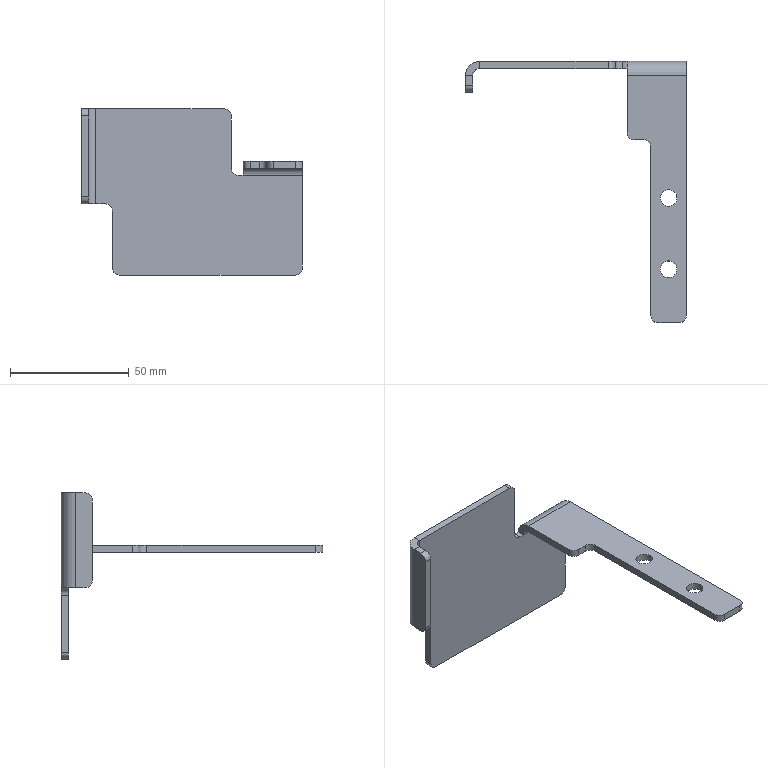Part | NX | features BREP 1 | 1 solid | 40 faces | box 93 x 110 x 70 mm | volume 22568 mm3 | plane 23 | cylinder 17 | commonest cylinder face diameters 6 x13 7 x2 12 x2
STEP:
#1=CARTESIAN_POINT('',(-17.5,-3.,-3.));
#2=VERTEX_POINT('',#1);
#3=CARTESIAN_POINT('',(-17.5,-3.,19.));
#4=VERTEX_POINT('',#3);
#5=CARTESIAN_POINT('',(-17.5,-3.,22.));
#6=DIRECTION('',(0.,0.,1.));
#7=VECTOR('',#6,1000.);
#8=LINE('',#5,#7);
#9=EDGE_CURVE('',#2,#4,#8,.T.);
#10=ORIENTED_EDGE('',*,*,#9,.T.);
#11=CARTESIAN_POINT('',(-20.5,-3.,22.));
#12=VERTEX_POINT('',#11);
#13=CARTESIAN_POINT('',(-20.5,-3.,19.));
#14=DIRECTION('',(0.,-1.,0.));
#15=DIRECTION('',(0.,0.,1.));
#16=AXIS2_PLACEMENT_3D('',#13,#14,#15);
#17=CIRCLE('',#16,3.);
#18=EDGE_CURVE('',#4,#12,#17,.T.);
#19=ORIENTED_EDGE('',*,*,#18,.T.);
#20=CARTESIAN_POINT('',(-74.5,-3.,22.));
#21=VERTEX_POINT('',#20);
#22=CARTESIAN_POINT('',(-77.5,-3.,22.));
#23=DIRECTION('',(-1.,0.,0.));
#24=VECTOR('',#23,1000.);
#25=LINE('',#22,#24);
#26=EDGE_CURVE('',#12,#21,#25,.T.);
#27=ORIENTED_EDGE('',*,*,#26,.T.);
#28=CARTESIAN_POINT('',(-74.5,-3.,-18.));
#29=VERTEX_POINT('',#28);
#30=CARTESIAN_POINT('',(-74.5,-3.,-48.));
#31=DIRECTION('',(0.,0.,1.));
#32=VECTOR('',#31,1000.);
#33=LINE('',#30,#32);
#34=EDGE_CURVE('',#29,#21,#33,.T.);
#35=ORIENTED_EDGE('',*,*,#34,.F.);
#36=CARTESIAN_POINT('',(-70.5,-3.,-18.));
#37=VERTEX_POINT('',#36);
#38=CARTESIAN_POINT('',(12.5,-3.,-18.));
#39=DIRECTION('',(1.,0.,0.));
#40=VECTOR('',#39,1000.);
#41=LINE('',#38,#40);
#42=EDGE_CURVE('',#29,#37,#41,.T.);
#43=ORIENTED_EDGE('',*,*,#42,.T.);
#44=CARTESIAN_POINT('',(-67.5,-3.,-21.));
#45=VERTEX_POINT('',#44);
#46=CARTESIAN_POINT('',(-70.5,-3.,-21.));
#47=DIRECTION('',(0.,1.,0.));
#48=DIRECTION('',(0.,0.,1.));
#49=AXIS2_PLACEMENT_3D('',#46,#47,#48);
#50=CIRCLE('',#49,3.);
#51=EDGE_CURVE('',#37,#45,#50,.T.);
#52=ORIENTED_EDGE('',*,*,#51,.T.);
#53=CARTESIAN_POINT('',(-67.5,-3.,-45.));
#54=VERTEX_POINT('',#53);
#55=CARTESIAN_POINT('',(-67.5,-3.,0.));
#56=DIRECTION('',(0.,0.,-1.));
#57=VECTOR('',#56,1000.);
#58=LINE('',#55,#57);
#59=EDGE_CURVE('',#45,#54,#58,.T.);
#60=ORIENTED_EDGE('',*,*,#59,.T.);
#61=CARTESIAN_POINT('',(-64.5,-3.,-48.));
#62=VERTEX_POINT('',#61);
#63=CARTESIAN_POINT('',(-64.5,-3.,-45.));
#64=DIRECTION('',(0.,-1.,0.));
#65=DIRECTION('',(0.,0.,1.));
#66=AXIS2_PLACEMENT_3D('',#63,#64,#65);
#67=CIRCLE('',#66,3.);
#68=EDGE_CURVE('',#54,#62,#67,.T.);
#69=ORIENTED_EDGE('',*,*,#68,.T.);
#70=CARTESIAN_POINT('',(9.5,-3.,-48.));
#71=VERTEX_POINT('',#70);
#72=CARTESIAN_POINT('',(12.5,-3.,-48.));
#73=DIRECTION('',(-1.,0.,0.));
#74=VECTOR('',#73,1000.);
#75=LINE('',#72,#74);
#76=EDGE_CURVE('',#71,#62,#75,.T.);
#77=ORIENTED_EDGE('',*,*,#76,.F.);
#78=CARTESIAN_POINT('',(12.5,-3.,-45.));
#79=VERTEX_POINT('',#78);
#80=CARTESIAN_POINT('',(9.5,-3.,-45.));
#81=DIRECTION('',(0.,-1.,0.));
#82=DIRECTION('',(0.,0.,1.));
#83=AXIS2_PLACEMENT_3D('',#80,#81,#82);
#84=CIRCLE('',#83,3.);
#85=EDGE_CURVE('',#71,#79,#84,.T.);
#86=ORIENTED_EDGE('',*,*,#85,.T.);
#87=CARTESIAN_POINT('',(12.5,-3.,-6.));
#88=VERTEX_POINT('',#87);
#89=CARTESIAN_POINT('',(12.5,-3.,0.));
#90=DIRECTION('',(0.,0.,-1.));
#91=VECTOR('',#90,1000.);
#92=LINE('',#89,#91);
#93=EDGE_CURVE('',#88,#79,#92,.T.);
#94=ORIENTED_EDGE('',*,*,#93,.F.);
#95=CARTESIAN_POINT('',(-12.5,-3.,-6.));
#96=VERTEX_POINT('',#95);
#97=CARTESIAN_POINT('',(12.5,-3.,-6.));
#98=DIRECTION('',(-1.,0.,0.));
#99=VECTOR('',#98,1000.);
#100=LINE('',#97,#99);
#101=EDGE_CURVE('',#88,#96,#100,.T.);
#102=ORIENTED_EDGE('',*,*,#101,.T.);
#103=CARTESIAN_POINT('',(-14.5,-3.,-6.));
#104=VERTEX_POINT('',#103);
#105=CARTESIAN_POINT('',(-17.5,-3.,-6.));
#106=DIRECTION('',(-1.,0.,0.));
#107=VECTOR('',#106,1000.);
#108=LINE('',#105,#107);
#109=EDGE_CURVE('',#96,#104,#108,.T.);
#110=ORIENTED_EDGE('',*,*,#109,.T.);
#111=CARTESIAN_POINT('',(-14.5,-3.,-3.));
#112=DIRECTION('',(0.,1.,0.));
#113=DIRECTION('',(0.,0.,1.));
#114=AXIS2_PLACEMENT_3D('',#111,#112,#113);
#115=CIRCLE('',#114,3.);
#116=EDGE_CURVE('',#104,#2,#115,.T.);
#117=ORIENTED_EDGE('',*,*,#116,.T.);
#118=EDGE_LOOP('',(#10,#19,#27,#35,#43,#52,#60,#69,#77,#86,#94,#102,#110,#117));
#119=FACE_BOUND('',#118,.T.);
#120=CARTESIAN_POINT('',(12.5,-3.,0.));
#121=DIRECTION('',(0.,1.,0.));
#122=DIRECTION('',(0.,0.,-1.));
#123=AXIS2_PLACEMENT_3D('',#120,#121,#122);
#124=PLANE('',#123);
#125=ADVANCED_FACE('',(#119),#124,.F.);
#126=CARTESIAN_POINT('',(9.5,0.,-48.));
#127=VERTEX_POINT('',#126);
#128=CARTESIAN_POINT('',(-64.5,0.,-48.));
#129=VERTEX_POINT('',#128);
#130=CARTESIAN_POINT('',(12.5,0.,-48.));
#131=DIRECTION('',(-1.,0.,0.));
#132=VECTOR('',#131,1000.);
#133=LINE('',#130,#132);
#134=EDGE_CURVE('',#127,#129,#133,.T.);
#135=ORIENTED_EDGE('',*,*,#134,.F.);
#136=CARTESIAN_POINT('',(9.5,0.,-48.));
#137=DIRECTION('',(0.,-1.,0.));
#138=VECTOR('',#137,1000.);
#139=LINE('',#136,#138);
#140=EDGE_CURVE('',#127,#71,#139,.T.);
#141=ORIENTED_EDGE('',*,*,#140,.T.);
#142=ORIENTED_EDGE('',*,*,#76,.T.);
#143=CARTESIAN_POINT('',(-64.5,0.,-48.));
#144=DIRECTION('',(0.,1.,0.));
#145=VECTOR('',#144,1000.);
#146=LINE('',#143,#145);
#147=EDGE_CURVE('',#62,#129,#146,.T.);
#148=ORIENTED_EDGE('',*,*,#147,.T.);
#149=EDGE_LOOP('',(#135,#141,#142,#148));
#150=FACE_BOUND('',#149,.T.);
#151=CARTESIAN_POINT('',(12.5,0.,-48.));
#152=DIRECTION('',(0.,0.,-1.));
#153=DIRECTION('',(1.,0.,0.));
#154=AXIS2_PLACEMENT_3D('',#151,#152,#153);
#155=PLANE('',#154);
#156=ADVANCED_FACE('',(#150),#155,.T.);
#157=CARTESIAN_POINT('',(-74.5,0.,22.));
#158=VERTEX_POINT('',#157);
#159=CARTESIAN_POINT('',(-20.5,0.,22.));
#160=VERTEX_POINT('',#159);
#161=CARTESIAN_POINT('',(-77.5,0.,22.));
#162=DIRECTION('',(1.,0.,0.));
#163=VECTOR('',#162,1000.);
#164=LINE('',#161,#163);
#165=EDGE_CURVE('',#158,#160,#164,.T.);
#166=ORIENTED_EDGE('',*,*,#165,.T.);
#167=CARTESIAN_POINT('',(-17.5,0.,19.));
#168=VERTEX_POINT('',#167);
#169=CARTESIAN_POINT('',(-20.5,0.,19.));
#170=DIRECTION('',(0.,1.,0.));
#171=DIRECTION('',(0.,0.,1.));
#172=AXIS2_PLACEMENT_3D('',#169,#170,#171);
#173=CIRCLE('',#172,3.);
#174=EDGE_CURVE('',#160,#168,#173,.T.);
#175=ORIENTED_EDGE('',*,*,#174,.T.);
#176=CARTESIAN_POINT('',(-17.5,0.,-3.));
#177=VERTEX_POINT('',#176);
#178=CARTESIAN_POINT('',(-17.5,0.,22.));
#179=DIRECTION('',(0.,0.,-1.));
#180=VECTOR('',#179,1000.);
#181=LINE('',#178,#180);
#182=EDGE_CURVE('',#168,#177,#181,.T.);
#183=ORIENTED_EDGE('',*,*,#182,.T.);
#184=CARTESIAN_POINT('',(-14.5,0.,-6.));
#185=VERTEX_POINT('',#184);
#186=CARTESIAN_POINT('',(-14.5,0.,-3.));
#187=DIRECTION('',(0.,-1.,0.));
#188=DIRECTION('',(0.,0.,1.));
#189=AXIS2_PLACEMENT_3D('',#186,#187,#188);
#190=CIRCLE('',#189,3.);
#191=EDGE_CURVE('',#177,#185,#190,.T.);
#192=ORIENTED_EDGE('',*,*,#191,.T.);
#193=CARTESIAN_POINT('',(-12.5,0.,-6.));
#194=VERTEX_POINT('',#193);
#195=CARTESIAN_POINT('',(-17.5,0.,-6.));
#196=DIRECTION('',(1.,0.,0.));
#197=VECTOR('',#196,1000.);
#198=LINE('',#195,#197);
#199=EDGE_CURVE('',#185,#194,#198,.T.);
#200=ORIENTED_EDGE('',*,*,#199,.T.);
#201=CARTESIAN_POINT('',(12.5,0.,-6.));
#202=VERTEX_POINT('',#201);
#203=CARTESIAN_POINT('',(12.5,0.,-6.));
#204=DIRECTION('',(-1.,0.,0.));
#205=VECTOR('',#204,1000.);
#206=LINE('',#203,#205);
#207=EDGE_CURVE('',#202,#194,#206,.T.);
#208=ORIENTED_EDGE('',*,*,#207,.F.);
#209=CARTESIAN_POINT('',(12.5,0.,-45.));
#210=VERTEX_POINT('',#209);
#211=CARTESIAN_POINT('',(12.5,0.,0.));
#212=DIRECTION('',(0.,0.,-1.));
#213=VECTOR('',#212,1000.);
#214=LINE('',#211,#213);
#215=EDGE_CURVE('',#202,#210,#214,.T.);
#216=ORIENTED_EDGE('',*,*,#215,.T.);
#217=CARTESIAN_POINT('',(9.5,0.,-45.));
#218=DIRECTION('',(0.,1.,0.));
#219=DIRECTION('',(0.,0.,1.));
#220=AXIS2_PLACEMENT_3D('',#217,#218,#219);
#221=CIRCLE('',#220,3.);
#222=EDGE_CURVE('',#210,#127,#221,.T.);
#223=ORIENTED_EDGE('',*,*,#222,.T.);
#224=ORIENTED_EDGE('',*,*,#134,.T.);
#225=CARTESIAN_POINT('',(-67.5,0.,-45.));
#226=VERTEX_POINT('',#225);
#227=CARTESIAN_POINT('',(-64.5,0.,-45.));
#228=DIRECTION('',(0.,1.,0.));
#229=DIRECTION('',(0.,0.,1.));
#230=AXIS2_PLACEMENT_3D('',#227,#228,#229);
#231=CIRCLE('',#230,3.);
#232=EDGE_CURVE('',#129,#226,#231,.T.);
#233=ORIENTED_EDGE('',*,*,#232,.T.);
#234=CARTESIAN_POINT('',(-67.5,0.,-21.));
#235=VERTEX_POINT('',#234);
#236=CARTESIAN_POINT('',(-67.5,0.,-48.));
#237=DIRECTION('',(0.,0.,-1.));
#238=VECTOR('',#237,1000.);
#239=LINE('',#236,#238);
#240=EDGE_CURVE('',#235,#226,#239,.T.);
#241=ORIENTED_EDGE('',*,*,#240,.F.);
#242=CARTESIAN_POINT('',(-70.5,0.,-18.));
#243=VERTEX_POINT('',#242);
#244=CARTESIAN_POINT('',(-70.5,0.,-21.));
#245=DIRECTION('',(0.,-1.,0.));
#246=DIRECTION('',(0.,0.,1.));
#247=AXIS2_PLACEMENT_3D('',#244,#245,#246);
#248=CIRCLE('',#247,3.);
#249=EDGE_CURVE('',#235,#243,#248,.T.);
#250=ORIENTED_EDGE('',*,*,#249,.T.);
#251=CARTESIAN_POINT('',(-74.5,0.,-18.));
#252=VERTEX_POINT('',#251);
#253=CARTESIAN_POINT('',(-67.5,0.,-18.));
#254=DIRECTION('',(1.,0.,0.));
#255=VECTOR('',#254,1000.);
#256=LINE('',#253,#255);
#257=EDGE_CURVE('',#252,#243,#256,.T.);
#258=ORIENTED_EDGE('',*,*,#257,.F.);
#259=CARTESIAN_POINT('',(-74.5,0.,-48.));
#260=DIRECTION('',(0.,0.,1.));
#261=VECTOR('',#260,1000.);
#262=LINE('',#259,#261);
#263=EDGE_CURVE('',#252,#158,#262,.T.);
#264=ORIENTED_EDGE('',*,*,#263,.T.);
#265=EDGE_LOOP('',(#166,#175,#183,#192,#200,#208,#216,#223,#224,#233,#241,#250,#258,#264));
#266=FACE_BOUND('',#265,.T.);
#267=CARTESIAN_POINT('',(12.5,0.,0.));
#268=DIRECTION('',(0.,1.,0.));
#269=DIRECTION('',(0.,0.,-1.));
#270=AXIS2_PLACEMENT_3D('',#267,#268,#269);
#271=PLANE('',#270);
#272=ADVANCED_FACE('',(#266),#271,.T.);
#273=CARTESIAN_POINT('',(12.5,0.,-6.));
#274=DIRECTION('',(0.,-1.,0.));
#275=VECTOR('',#274,1000.);
#276=LINE('',#273,#275);
#277=EDGE_CURVE('',#202,#88,#276,.T.);
#278=ORIENTED_EDGE('',*,*,#277,.F.);
#279=CARTESIAN_POINT('',(12.5,-6.,0.));
#280=VERTEX_POINT('',#279);
#281=CARTESIAN_POINT('',(12.5,-6.,-6.));
#282=DIRECTION('',(-1.,0.,0.));
#283=DIRECTION('',(0.,0.,-1.));
#284=AXIS2_PLACEMENT_3D('',#281,#282,#283);
#285=CIRCLE('',#284,6.);
#286=EDGE_CURVE('',#280,#202,#285,.T.);
#287=ORIENTED_EDGE('',*,*,#286,.F.);
#288=CARTESIAN_POINT('',(12.5,-6.,-3.));
#289=VERTEX_POINT('',#288);
#290=CARTESIAN_POINT('',(12.5,-6.,-3.));
#291=DIRECTION('',(0.,0.,1.));
#292=VECTOR('',#291,1000.);
#293=LINE('',#290,#292);
#294=EDGE_CURVE('',#289,#280,#293,.T.);
#295=ORIENTED_EDGE('',*,*,#294,.F.);
#296=CARTESIAN_POINT('',(12.5,-6.,-6.));
#297=DIRECTION('',(-1.,0.,0.));
#298=DIRECTION('',(0.,0.,-1.));
#299=AXIS2_PLACEMENT_3D('',#296,#297,#298);
#300=CIRCLE('',#299,3.);
#301=EDGE_CURVE('',#289,#88,#300,.T.);
#302=ORIENTED_EDGE('',*,*,#301,.T.);
#303=EDGE_LOOP('',(#278,#287,#295,#302));
#304=FACE_BOUND('',#303,.T.);
#305=CARTESIAN_POINT('',(12.5,0.,-6.));
#306=DIRECTION('',(1.,0.,0.));
#307=DIRECTION('',(0.,0.,1.));
#308=AXIS2_PLACEMENT_3D('',#305,#306,#307);
#309=PLANE('',#308);
#310=ADVANCED_FACE('',(#304),#309,.T.);
#311=ORIENTED_EDGE('',*,*,#93,.T.);
#312=CARTESIAN_POINT('',(12.5,-6.,-45.));
#313=DIRECTION('',(0.,1.,0.));
#314=VECTOR('',#313,1000.);
#315=LINE('',#312,#314);
#316=EDGE_CURVE('',#79,#210,#315,.T.);
#317=ORIENTED_EDGE('',*,*,#316,.T.);
#318=ORIENTED_EDGE('',*,*,#215,.F.);
#319=ORIENTED_EDGE('',*,*,#277,.T.);
#320=EDGE_LOOP('',(#311,#317,#318,#319));
#321=FACE_BOUND('',#320,.T.);
#322=CARTESIAN_POINT('',(12.5,-6.,-3.));
#323=DIRECTION('',(1.,0.,0.));
#324=DIRECTION('',(0.,0.,1.));
#325=AXIS2_PLACEMENT_3D('',#322,#323,#324);
#326=PLANE('',#325);
#327=ADVANCED_FACE('',(#321),#326,.T.);
#328=CARTESIAN_POINT('',(-12.5,-6.,0.));
#329=VERTEX_POINT('',#328);
#330=CARTESIAN_POINT('',(-12.5,-6.,-3.));
#331=VERTEX_POINT('',#330);
#332=CARTESIAN_POINT('',(-12.5,-6.,0.));
#333=DIRECTION('',(0.,0.,-1.));
#334=VECTOR('',#333,1000.);
#335=LINE('',#332,#334);
#336=EDGE_CURVE('',#329,#331,#335,.T.);
#337=ORIENTED_EDGE('',*,*,#336,.F.);
#338=CARTESIAN_POINT('',(-12.5,-6.,-6.));
#339=DIRECTION('',(-1.,0.,0.));
#340=DIRECTION('',(0.,0.,-1.));
#341=AXIS2_PLACEMENT_3D('',#338,#339,#340);
#342=CIRCLE('',#341,6.);
#343=EDGE_CURVE('',#329,#194,#342,.T.);
#344=ORIENTED_EDGE('',*,*,#343,.T.);
#345=CARTESIAN_POINT('',(-12.5,-3.,-6.));
#346=DIRECTION('',(0.,1.,0.));
#347=VECTOR('',#346,1000.);
#348=LINE('',#345,#347);
#349=EDGE_CURVE('',#96,#194,#348,.T.);
#350=ORIENTED_EDGE('',*,*,#349,.F.);
#351=CARTESIAN_POINT('',(-12.5,-6.,-6.));
#352=DIRECTION('',(-1.,0.,0.));
#353=DIRECTION('',(0.,0.,-1.));
#354=AXIS2_PLACEMENT_3D('',#351,#352,#353);
#355=CIRCLE('',#354,3.);
#356=EDGE_CURVE('',#331,#96,#355,.T.);
#357=ORIENTED_EDGE('',*,*,#356,.F.);
#358=EDGE_LOOP('',(#337,#344,#350,#357));
#359=FACE_BOUND('',#358,.T.);
#360=CARTESIAN_POINT('',(-12.5,-6.,0.));
#361=DIRECTION('',(-1.,0.,0.));
#362=DIRECTION('',(0.,0.,-1.));
#363=AXIS2_PLACEMENT_3D('',#360,#361,#362);
#364=PLANE('',#363);
#365=ADVANCED_FACE('',(#359),#364,.T.);
#366=CARTESIAN_POINT('',(-12.5,-30.,-3.));
#367=VERTEX_POINT('',#366);
#368=CARTESIAN_POINT('',(-12.5,-110.,-3.));
#369=DIRECTION('',(0.,1.,0.));
#370=VECTOR('',#369,1000.);
#371=LINE('',#368,#370);
#372=EDGE_CURVE('',#367,#331,#371,.T.);
#373=ORIENTED_EDGE('',*,*,#372,.F.);
#374=CARTESIAN_POINT('',(-12.5,-30.,0.));
#375=VERTEX_POINT('',#374);
#376=CARTESIAN_POINT('',(-12.5,-30.,0.));
#377=DIRECTION('',(0.,0.,1.));
#378=VECTOR('',#377,1000.);
#379=LINE('',#376,#378);
#380=EDGE_CURVE('',#367,#375,#379,.T.);
#381=ORIENTED_EDGE('',*,*,#380,.T.);
#382=CARTESIAN_POINT('',(-12.5,-110.,0.));
#383=DIRECTION('',(0.,1.,0.));
#384=VECTOR('',#383,1000.);
#385=LINE('',#382,#384);
#386=EDGE_CURVE('',#375,#329,#385,.T.);
#387=ORIENTED_EDGE('',*,*,#386,.T.);
#388=ORIENTED_EDGE('',*,*,#336,.T.);
#389=EDGE_LOOP('',(#373,#381,#387,#388));
#390=FACE_BOUND('',#389,.T.);
#391=CARTESIAN_POINT('',(-12.5,-3.,-6.));
#392=DIRECTION('',(-1.,0.,0.));
#393=DIRECTION('',(0.,0.,-1.));
#394=AXIS2_PLACEMENT_3D('',#391,#392,#393);
#395=PLANE('',#394);
#396=ADVANCED_FACE('',(#390),#395,.T.);
#397=ORIENTED_EDGE('',*,*,#343,.F.);
#398=CARTESIAN_POINT('',(12.5,-6.,0.));
#399=DIRECTION('',(-1.,0.,0.));
#400=VECTOR('',#399,1000.);
#401=LINE('',#398,#400);
#402=EDGE_CURVE('',#280,#329,#401,.T.);
#403=ORIENTED_EDGE('',*,*,#402,.F.);
#404=ORIENTED_EDGE('',*,*,#286,.T.);
#405=ORIENTED_EDGE('',*,*,#207,.T.);
#406=EDGE_LOOP('',(#397,#403,#404,#405));
#407=FACE_BOUND('',#406,.T.);
#408=CARTESIAN_POINT('',(12.5,-6.,-6.));
#409=DIRECTION('',(-1.,0.,0.));
#410=DIRECTION('',(0.,0.,-1.));
#411=AXIS2_PLACEMENT_3D('',#408,#409,#410);
#412=CYLINDRICAL_SURFACE('',#411,6.);
#413=ADVANCED_FACE('',(#407),#412,.T.);
#414=CARTESIAN_POINT('',(8.5,-57.5,0.));
#415=VERTEX_POINT('',#414);
#416=CARTESIAN_POINT('',(5.,-57.5,0.));
#417=DIRECTION('',(0.,0.,1.));
#418=DIRECTION('',(1.,0.,0.));
#419=AXIS2_PLACEMENT_3D('',#416,#417,#418);
#420=CIRCLE('',#419,3.5);
#421=EDGE_CURVE('',#415,#415,#420,.T.);
#422=ORIENTED_EDGE('',*,*,#421,.F.);
#423=EDGE_LOOP('',(#422));
#424=FACE_BOUND('',#423,.T.);
#425=CARTESIAN_POINT('',(8.5,-87.5,0.));
#426=VERTEX_POINT('',#425);
#427=CARTESIAN_POINT('',(5.,-87.5,0.));
#428=DIRECTION('',(0.,0.,1.));
#429=DIRECTION('',(1.,0.,0.));
#430=AXIS2_PLACEMENT_3D('',#427,#428,#429);
#431=CIRCLE('',#430,3.5);
#432=EDGE_CURVE('',#426,#426,#431,.T.);
#433=ORIENTED_EDGE('',*,*,#432,.F.);
#434=EDGE_LOOP('',(#433));
#435=FACE_BOUND('',#434,.T.);
#436=CARTESIAN_POINT('',(9.5,-110.,0.));
#437=VERTEX_POINT('',#436);
#438=CARTESIAN_POINT('',(0.5,-110.,0.));
#439=VERTEX_POINT('',#438);
#440=CARTESIAN_POINT('',(12.5,-110.,0.));
#441=DIRECTION('',(-1.,0.,0.));
#442=VECTOR('',#441,1000.);
#443=LINE('',#440,#442);
#444=EDGE_CURVE('',#437,#439,#443,.T.);
#445=ORIENTED_EDGE('',*,*,#444,.F.);
#446=CARTESIAN_POINT('',(12.5,-107.,0.));
#447=VERTEX_POINT('',#446);
#448=CARTESIAN_POINT('',(9.5,-107.,0.));
#449=DIRECTION('',(0.,0.,1.));
#450=DIRECTION('',(1.,0.,0.));
#451=AXIS2_PLACEMENT_3D('',#448,#449,#450);
#452=CIRCLE('',#451,3.);
#453=EDGE_CURVE('',#437,#447,#452,.T.);
#454=ORIENTED_EDGE('',*,*,#453,.T.);
#455=CARTESIAN_POINT('',(12.5,-110.,0.));
#456=DIRECTION('',(0.,1.,0.));
#457=VECTOR('',#456,1000.);
#458=LINE('',#455,#457);
#459=EDGE_CURVE('',#447,#280,#458,.T.);
#460=ORIENTED_EDGE('',*,*,#459,.T.);
#461=ORIENTED_EDGE('',*,*,#402,.T.);
#462=ORIENTED_EDGE('',*,*,#386,.F.);
#463=CARTESIAN_POINT('',(-9.5,-33.,0.));
#464=VERTEX_POINT('',#463);
#465=CARTESIAN_POINT('',(-9.5,-30.,0.));
#466=DIRECTION('',(0.,0.,1.));
#467=DIRECTION('',(1.,0.,0.));
#468=AXIS2_PLACEMENT_3D('',#465,#466,#467);
#469=CIRCLE('',#468,3.);
#470=EDGE_CURVE('',#375,#464,#469,.T.);
#471=ORIENTED_EDGE('',*,*,#470,.T.);
#472=CARTESIAN_POINT('',(-5.5,-33.,0.));
#473=VERTEX_POINT('',#472);
#474=CARTESIAN_POINT('',(-12.5,-33.,0.));
#475=DIRECTION('',(-1.,0.,0.));
#476=VECTOR('',#475,1000.);
#477=LINE('',#474,#476);
#478=EDGE_CURVE('',#473,#464,#477,.T.);
#479=ORIENTED_EDGE('',*,*,#478,.F.);
#480=CARTESIAN_POINT('',(-2.5,-36.,0.));
#481=VERTEX_POINT('',#480);
#482=CARTESIAN_POINT('',(-5.5,-36.,0.));
#483=DIRECTION('',(0.,0.,-1.));
#484=DIRECTION('',(1.,0.,0.));
#485=AXIS2_PLACEMENT_3D('',#482,#483,#484);
#486=CIRCLE('',#485,3.);
#487=EDGE_CURVE('',#473,#481,#486,.T.);
#488=ORIENTED_EDGE('',*,*,#487,.T.);
#489=CARTESIAN_POINT('',(-2.5,-107.,0.));
#490=VERTEX_POINT('',#489);
#491=CARTESIAN_POINT('',(-2.5,-110.,0.));
#492=DIRECTION('',(0.,1.,0.));
#493=VECTOR('',#492,1000.);
#494=LINE('',#491,#493);
#495=EDGE_CURVE('',#490,#481,#494,.T.);
#496=ORIENTED_EDGE('',*,*,#495,.F.);
#497=CARTESIAN_POINT('',(0.5,-107.,0.));
#498=DIRECTION('',(0.,0.,1.));
#499=DIRECTION('',(1.,0.,0.));
#500=AXIS2_PLACEMENT_3D('',#497,#498,#499);
#501=CIRCLE('',#500,3.);
#502=EDGE_CURVE('',#490,#439,#501,.T.);
#503=ORIENTED_EDGE('',*,*,#502,.T.);
#504=EDGE_LOOP('',(#445,#454,#460,#461,#462,#471,#479,#488,#496,#503));
#505=FACE_BOUND('',#504,.T.);
#506=CARTESIAN_POINT('',(12.5,-110.,0.));
#507=DIRECTION('',(0.,0.,1.));
#508=DIRECTION('',(-1.,0.,0.));
#509=AXIS2_PLACEMENT_3D('',#506,#507,#508);
#510=PLANE('',#509);
#511=ADVANCED_FACE('',(#424,#435,#505),#510,.T.);
#512=CARTESIAN_POINT('',(9.5,-110.,-3.));
#513=VERTEX_POINT('',#512);
#514=CARTESIAN_POINT('',(0.5,-110.,-3.));
#515=VERTEX_POINT('',#514);
#516=CARTESIAN_POINT('',(12.5,-110.,-3.));
#517=DIRECTION('',(-1.,0.,0.));
#518=VECTOR('',#517,1000.);
#519=LINE('',#516,#518);
#520=EDGE_CURVE('',#513,#515,#519,.T.);
#521=ORIENTED_EDGE('',*,*,#520,.F.);
#522=CARTESIAN_POINT('',(9.5,-110.,-3.));
#523=DIRECTION('',(0.,0.,1.));
#524=VECTOR('',#523,1000.);
#525=LINE('',#522,#524);
#526=EDGE_CURVE('',#513,#437,#525,.T.);
#527=ORIENTED_EDGE('',*,*,#526,.T.);
#528=ORIENTED_EDGE('',*,*,#444,.T.);
#529=CARTESIAN_POINT('',(0.5,-110.,-3.));
#530=DIRECTION('',(0.,0.,-1.));
#531=VECTOR('',#530,1000.);
#532=LINE('',#529,#531);
#533=EDGE_CURVE('',#439,#515,#532,.T.);
#534=ORIENTED_EDGE('',*,*,#533,.T.);
#535=EDGE_LOOP('',(#521,#527,#528,#534));
#536=FACE_BOUND('',#535,.T.);
#537=CARTESIAN_POINT('',(12.5,-110.,-3.));
#538=DIRECTION('',(0.,-1.,0.));
#539=DIRECTION('',(0.,0.,1.));
#540=AXIS2_PLACEMENT_3D('',#537,#538,#539);
#541=PLANE('',#540);
#542=ADVANCED_FACE('',(#536),#541,.T.);
#543=CARTESIAN_POINT('',(8.5,-57.5,-3.));
#544=VERTEX_POINT('',#543);
#545=CARTESIAN_POINT('',(5.,-57.5,-3.));
#546=DIRECTION('',(0.,0.,1.));
#547=DIRECTION('',(1.,0.,0.));
#548=AXIS2_PLACEMENT_3D('',#545,#546,#547);
#549=CIRCLE('',#548,3.5);
#550=EDGE_CURVE('',#544,#544,#549,.T.);
#551=ORIENTED_EDGE('',*,*,#550,.T.);
#552=EDGE_LOOP('',(#551));
#553=FACE_BOUND('',#552,.T.);
#554=CARTESIAN_POINT('',(8.5,-87.5,-3.));
#555=VERTEX_POINT('',#554);
#556=CARTESIAN_POINT('',(5.,-87.5,-3.));
#557=DIRECTION('',(0.,0.,1.));
#558=DIRECTION('',(1.,0.,0.));
#559=AXIS2_PLACEMENT_3D('',#556,#557,#558);
#560=CIRCLE('',#559,3.5);
#561=EDGE_CURVE('',#555,#555,#560,.T.);
#562=ORIENTED_EDGE('',*,*,#561,.T.);
#563=EDGE_LOOP('',(#562));
#564=FACE_BOUND('',#563,.T.);
#565=CARTESIAN_POINT('',(12.5,-107.,-3.));
#566=VERTEX_POINT('',#565);
#567=CARTESIAN_POINT('',(12.5,-110.,-3.));
#568=DIRECTION('',(0.,1.,0.));
#569=VECTOR('',#568,1000.);
#570=LINE('',#567,#569);
#571=EDGE_CURVE('',#566,#289,#570,.T.);
#572=ORIENTED_EDGE('',*,*,#571,.F.);
#573=CARTESIAN_POINT('',(9.5,-107.,-3.));
#574=DIRECTION('',(0.,0.,-1.));
#575=DIRECTION('',(1.,0.,0.));
#576=AXIS2_PLACEMENT_3D('',#573,#574,#575);
#577=CIRCLE('',#576,3.);
#578=EDGE_CURVE('',#566,#513,#577,.T.);
#579=ORIENTED_EDGE('',*,*,#578,.T.);
#580=ORIENTED_EDGE('',*,*,#520,.T.);
#581=CARTESIAN_POINT('',(-2.5,-107.,-3.));
#582=VERTEX_POINT('',#581);
#583=CARTESIAN_POINT('',(0.5,-107.,-3.));
#584=DIRECTION('',(0.,0.,-1.));
#585=DIRECTION('',(1.,0.,0.));
#586=AXIS2_PLACEMENT_3D('',#583,#584,#585);
#587=CIRCLE('',#586,3.);
#588=EDGE_CURVE('',#515,#582,#587,.T.);
#589=ORIENTED_EDGE('',*,*,#588,.T.);
#590=CARTESIAN_POINT('',(-2.5,-36.,-3.));
#591=VERTEX_POINT('',#590);
#592=CARTESIAN_POINT('',(-2.5,-110.,-3.));
#593=DIRECTION('',(0.,-1.,0.));
#594=VECTOR('',#593,1000.);
#595=LINE('',#592,#594);
#596=EDGE_CURVE('',#591,#582,#595,.T.);
#597=ORIENTED_EDGE('',*,*,#596,.F.);
#598=CARTESIAN_POINT('',(-5.5,-33.,-3.));
#599=VERTEX_POINT('',#598);
#600=CARTESIAN_POINT('',(-5.5,-36.,-3.));
#601=DIRECTION('',(0.,0.,1.));
#602=DIRECTION('',(1.,0.,0.));
#603=AXIS2_PLACEMENT_3D('',#600,#601,#602);
#604=CIRCLE('',#603,3.);
#605=EDGE_CURVE('',#591,#599,#604,.T.);
#606=ORIENTED_EDGE('',*,*,#605,.T.);
#607=CARTESIAN_POINT('',(-9.5,-33.,-3.));
#608=VERTEX_POINT('',#607);
#609=CARTESIAN_POINT('',(-12.5,-33.,-3.));
#610=DIRECTION('',(1.,0.,0.));
#611=VECTOR('',#610,1000.);
#612=LINE('',#609,#611);
#613=EDGE_CURVE('',#608,#599,#612,.T.);
#614=ORIENTED_EDGE('',*,*,#613,.F.);
#615=CARTESIAN_POINT('',(-9.5,-30.,-3.));
#616=DIRECTION('',(0.,0.,-1.));
#617=DIRECTION('',(1.,0.,0.));
#618=AXIS2_PLACEMENT_3D('',#615,#616,#617);
#619=CIRCLE('',#618,3.);
#620=EDGE_CURVE('',#608,#367,#619,.T.);
#621=ORIENTED_EDGE('',*,*,#620,.T.);
#622=ORIENTED_EDGE('',*,*,#372,.T.);
#623=CARTESIAN_POINT('',(12.5,-6.,-3.));
#624=DIRECTION('',(-1.,0.,0.));
#625=VECTOR('',#624,1000.);
#626=LINE('',#623,#625);
#627=EDGE_CURVE('',#289,#331,#626,.T.);
#628=ORIENTED_EDGE('',*,*,#627,.F.);
#629=EDGE_LOOP('',(#572,#579,#580,#589,#597,#606,#614,#621,#622,#628));
#630=FACE_BOUND('',#629,.T.);
#631=CARTESIAN_POINT('',(12.5,-110.,-3.));
#632=DIRECTION('',(0.,0.,1.));
#633=DIRECTION('',(-1.,0.,0.));
#634=AXIS2_PLACEMENT_3D('',#631,#632,#633);
#635=PLANE('',#634);
#636=ADVANCED_FACE('',(#553,#564,#630),#635,.F.);
#637=ORIENTED_EDGE('',*,*,#356,.T.);
#638=ORIENTED_EDGE('',*,*,#101,.F.);
#639=ORIENTED_EDGE('',*,*,#301,.F.);
#640=ORIENTED_EDGE('',*,*,#627,.T.);
#641=EDGE_LOOP('',(#637,#638,#639,#640));
#642=FACE_BOUND('',#641,.T.);
#643=CARTESIAN_POINT('',(12.5,-6.,-6.));
#644=DIRECTION('',(-1.,0.,0.));
#645=DIRECTION('',(0.,0.,-1.));
#646=AXIS2_PLACEMENT_3D('',#643,#644,#645);
#647=CYLINDRICAL_SURFACE('',#646,3.);
#648=ADVANCED_FACE('',(#642),#647,.F.);
#649=ORIENTED_EDGE('',*,*,#459,.F.);
#650=CARTESIAN_POINT('',(12.5,-107.,-6.));
#651=DIRECTION('',(0.,0.,-1.));
#652=VECTOR('',#651,1000.);
#653=LINE('',#650,#652);
#654=EDGE_CURVE('',#447,#566,#653,.T.);
#655=ORIENTED_EDGE('',*,*,#654,.T.);
#656=ORIENTED_EDGE('',*,*,#571,.T.);
#657=ORIENTED_EDGE('',*,*,#294,.T.);
#658=EDGE_LOOP('',(#649,#655,#656,#657));
#659=FACE_BOUND('',#658,.T.);
#660=CARTESIAN_POINT('',(12.5,-6.,-6.));
#661=DIRECTION('',(1.,0.,0.));
#662=DIRECTION('',(0.,0.,1.));
#663=AXIS2_PLACEMENT_3D('',#660,#661,#662);
#664=PLANE('',#663);
#665=ADVANCED_FACE('',(#659),#664,.T.);
#666=ORIENTED_EDGE('',*,*,#199,.F.);
#667=CARTESIAN_POINT('',(-14.5,-3.,-6.));
#668=DIRECTION('',(0.,-1.,0.));
#669=VECTOR('',#668,1000.);
#670=LINE('',#667,#669);
#671=EDGE_CURVE('',#185,#104,#670,.T.);
#672=ORIENTED_EDGE('',*,*,#671,.T.);
#673=ORIENTED_EDGE('',*,*,#109,.F.);
#674=ORIENTED_EDGE('',*,*,#349,.T.);
#675=EDGE_LOOP('',(#666,#672,#673,#674));
#676=FACE_BOUND('',#675,.T.);
#677=CARTESIAN_POINT('',(-17.5,-98.525,-6.));
#678=DIRECTION('',(0.,0.,1.));
#679=DIRECTION('',(-1.,0.,0.));
#680=AXIS2_PLACEMENT_3D('',#677,#678,#679);
#681=PLANE('',#680);
#682=ADVANCED_FACE('',(#676),#681,.T.);
#683=ORIENTED_EDGE('',*,*,#9,.F.);
#684=CARTESIAN_POINT('',(-17.5,0.,-3.));
#685=DIRECTION('',(0.,1.,0.));
#686=VECTOR('',#685,1000.);
#687=LINE('',#684,#686);
#688=EDGE_CURVE('',#2,#177,#687,.T.);
#689=ORIENTED_EDGE('',*,*,#688,.T.);
#690=ORIENTED_EDGE('',*,*,#182,.F.);
#691=CARTESIAN_POINT('',(-17.5,-98.525,19.));
#692=DIRECTION('',(0.,-1.,0.));
#693=VECTOR('',#692,1000.);
#694=LINE('',#691,#693);
#695=EDGE_CURVE('',#168,#4,#694,.T.);
#696=ORIENTED_EDGE('',*,*,#695,.T.);
#697=EDGE_LOOP('',(#683,#689,#690,#696));
#698=FACE_BOUND('',#697,.T.);
#699=CARTESIAN_POINT('',(-17.5,-98.525,22.));
#700=DIRECTION('',(1.,0.,0.));
#701=DIRECTION('',(0.,0.,1.));
#702=AXIS2_PLACEMENT_3D('',#699,#700,#701);
#703=PLANE('',#702);
#704=ADVANCED_FACE('',(#698),#703,.T.);
#705=ORIENTED_EDGE('',*,*,#26,.F.);
#706=CARTESIAN_POINT('',(-20.5,-98.525,22.));
#707=DIRECTION('',(0.,1.,0.));
#708=VECTOR('',#707,1000.);
#709=LINE('',#706,#708);
#710=EDGE_CURVE('',#12,#160,#709,.T.);
#711=ORIENTED_EDGE('',*,*,#710,.T.);
#712=ORIENTED_EDGE('',*,*,#165,.F.);
#713=CARTESIAN_POINT('',(-74.5,-3.,22.));
#714=DIRECTION('',(0.,1.,0.));
#715=VECTOR('',#714,1000.);
#716=LINE('',#713,#715);
#717=EDGE_CURVE('',#21,#158,#716,.T.);
#718=ORIENTED_EDGE('',*,*,#717,.F.);
#719=EDGE_LOOP('',(#705,#711,#712,#718));
#720=FACE_BOUND('',#719,.T.);
#721=CARTESIAN_POINT('',(-77.5,-98.525,22.));
#722=DIRECTION('',(0.,0.,1.));
#723=DIRECTION('',(-1.,0.,0.));
#724=AXIS2_PLACEMENT_3D('',#721,#722,#723);
#725=PLANE('',#724);
#726=ADVANCED_FACE('',(#720),#725,.T.);
#727=CARTESIAN_POINT('',(-77.5,-6.,22.));
#728=VERTEX_POINT('',#727);
#729=CARTESIAN_POINT('',(-80.5,-6.,22.));
#730=VERTEX_POINT('',#729);
#731=CARTESIAN_POINT('',(-77.5,-6.,22.));
#732=DIRECTION('',(-1.,0.,0.));
#733=VECTOR('',#732,1000.);
#734=LINE('',#731,#733);
#735=EDGE_CURVE('',#728,#730,#734,.T.);
#736=ORIENTED_EDGE('',*,*,#735,.F.);
#737=CARTESIAN_POINT('',(-74.5,-6.,22.));
#738=DIRECTION('',(0.,0.,1.));
#739=DIRECTION('',(-1.,0.,0.));
#740=AXIS2_PLACEMENT_3D('',#737,#738,#739);
#741=CIRCLE('',#740,3.);
#742=EDGE_CURVE('',#21,#728,#741,.T.);
#743=ORIENTED_EDGE('',*,*,#742,.F.);
#744=ORIENTED_EDGE('',*,*,#717,.T.);
#745=CARTESIAN_POINT('',(-74.5,-6.,22.));
#746=DIRECTION('',(0.,0.,1.));
#747=DIRECTION('',(-1.,0.,0.));
#748=AXIS2_PLACEMENT_3D('',#745,#746,#747);
#749=CIRCLE('',#748,6.);
#750=EDGE_CURVE('',#158,#730,#749,.T.);
#751=ORIENTED_EDGE('',*,*,#750,.T.);
#752=EDGE_LOOP('',(#736,#743,#744,#751));
#753=FACE_BOUND('',#752,.T.);
#754=CARTESIAN_POINT('',(-74.5,-6.,22.));
#755=DIRECTION('',(0.,0.,1.));
#756=DIRECTION('',(-1.,0.,0.));
#757=AXIS2_PLACEMENT_3D('',#754,#755,#756);
#758=PLANE('',#757);
#759=ADVANCED_FACE('',(#753),#758,.T.);
#760=CARTESIAN_POINT('',(-80.5,-6.,-18.));
#761=VERTEX_POINT('',#760);
#762=CARTESIAN_POINT('',(-74.5,-6.,-18.));
#763=DIRECTION('',(0.,0.,-1.));
#764=DIRECTION('',(1.,0.,0.));
#765=AXIS2_PLACEMENT_3D('',#762,#763,#764);
#766=CIRCLE('',#765,6.);
#767=EDGE_CURVE('',#761,#252,#766,.T.);
#768=ORIENTED_EDGE('',*,*,#767,.F.);
#769=CARTESIAN_POINT('',(-80.5,-6.,0.));
#770=DIRECTION('',(0.,0.,1.));
#771=VECTOR('',#770,1000.);
#772=LINE('',#769,#771);
#773=EDGE_CURVE('',#761,#730,#772,.T.);
#774=ORIENTED_EDGE('',*,*,#773,.T.);
#775=ORIENTED_EDGE('',*,*,#750,.F.);
#776=ORIENTED_EDGE('',*,*,#263,.F.);
#777=EDGE_LOOP('',(#768,#774,#775,#776));
#778=FACE_BOUND('',#777,.T.);
#779=CARTESIAN_POINT('',(-74.5,-6.,-48.));
#780=DIRECTION('',(0.,0.,-1.));
#781=DIRECTION('',(1.,0.,0.));
#782=AXIS2_PLACEMENT_3D('',#779,#780,#781);
#783=CYLINDRICAL_SURFACE('',#782,6.);
#784=ADVANCED_FACE('',(#778),#783,.T.);
#785=CARTESIAN_POINT('',(-77.5,-6.,-18.));
#786=VERTEX_POINT('',#785);
#787=CARTESIAN_POINT('',(-77.5,-6.,22.));
#788=DIRECTION('',(0.,0.,-1.));
#789=VECTOR('',#788,1000.);
#790=LINE('',#787,#789);
#791=EDGE_CURVE('',#728,#786,#790,.T.);
#792=ORIENTED_EDGE('',*,*,#791,.T.);
#793=CARTESIAN_POINT('',(-74.5,-6.,-18.));
#794=DIRECTION('',(0.,0.,-1.));
#795=DIRECTION('',(1.,0.,0.));
#796=AXIS2_PLACEMENT_3D('',#793,#794,#795);
#797=CIRCLE('',#796,3.);
#798=EDGE_CURVE('',#786,#29,#797,.T.);
#799=ORIENTED_EDGE('',*,*,#798,.T.);
#800=ORIENTED_EDGE('',*,*,#34,.T.);
#801=ORIENTED_EDGE('',*,*,#742,.T.);
#802=EDGE_LOOP('',(#792,#799,#800,#801));
#803=FACE_BOUND('',#802,.T.);
#804=CARTESIAN_POINT('',(-74.5,-6.,-48.));
#805=DIRECTION('',(0.,0.,-1.));
#806=DIRECTION('',(1.,0.,0.));
#807=AXIS2_PLACEMENT_3D('',#804,#805,#806);
#808=CYLINDRICAL_SURFACE('',#807,3.);
#809=ADVANCED_FACE('',(#803),#808,.F.);
#810=CARTESIAN_POINT('',(-80.5,-10.,22.));
#811=VERTEX_POINT('',#810);
#812=CARTESIAN_POINT('',(-80.5,-3.,22.));
#813=DIRECTION('',(0.,1.,0.));
#814=VECTOR('',#813,1000.);
#815=LINE('',#812,#814);
#816=EDGE_CURVE('',#811,#730,#815,.T.);
#817=ORIENTED_EDGE('',*,*,#816,.F.);
#818=CARTESIAN_POINT('',(-77.5,-10.,22.));
#819=VERTEX_POINT('',#818);
#820=CARTESIAN_POINT('',(-80.5,-10.,22.));
#821=DIRECTION('',(1.,0.,0.));
#822=VECTOR('',#821,1000.);
#823=LINE('',#820,#822);
#824=EDGE_CURVE('',#811,#819,#823,.T.);
#825=ORIENTED_EDGE('',*,*,#824,.T.);
#826=CARTESIAN_POINT('',(-77.5,-3.,22.));
#827=DIRECTION('',(0.,1.,0.));
#828=VECTOR('',#827,1000.);
#829=LINE('',#826,#828);
#830=EDGE_CURVE('',#819,#728,#829,.T.);
#831=ORIENTED_EDGE('',*,*,#830,.T.);
#832=ORIENTED_EDGE('',*,*,#735,.T.);
#833=EDGE_LOOP('',(#817,#825,#831,#832));
#834=FACE_BOUND('',#833,.T.);
#835=CARTESIAN_POINT('',(-80.5,-3.,22.));
#836=DIRECTION('',(0.,0.,-1.));
#837=DIRECTION('',(0.,-1.,0.));
#838=AXIS2_PLACEMENT_3D('',#835,#836,#837);
#839=PLANE('',#838);
#840=ADVANCED_FACE('',(#834),#839,.F.);
#841=CARTESIAN_POINT('',(-80.5,-13.,-15.));
#842=VERTEX_POINT('',#841);
#843=CARTESIAN_POINT('',(-80.5,-13.,19.));
#844=VERTEX_POINT('',#843);
#845=CARTESIAN_POINT('',(-80.5,-13.,22.));
#846=DIRECTION('',(0.,0.,1.));
#847=VECTOR('',#846,1000.);
#848=LINE('',#845,#847);
#849=EDGE_CURVE('',#842,#844,#848,.T.);
#850=ORIENTED_EDGE('',*,*,#849,.T.);
#851=CARTESIAN_POINT('',(-80.5,-10.,19.));
#852=DIRECTION('',(-1.,0.,0.));
#853=DIRECTION('',(0.,1.,0.));
#854=AXIS2_PLACEMENT_3D('',#851,#852,#853);
#855=CIRCLE('',#854,3.);
#856=EDGE_CURVE('',#844,#811,#855,.T.);
#857=ORIENTED_EDGE('',*,*,#856,.T.);
#858=ORIENTED_EDGE('',*,*,#816,.T.);
#859=ORIENTED_EDGE('',*,*,#773,.F.);
#860=CARTESIAN_POINT('',(-80.5,-10.,-18.));
#861=VERTEX_POINT('',#860);
#862=CARTESIAN_POINT('',(-80.5,-110.,-18.));
#863=DIRECTION('',(0.,1.,0.));
#864=VECTOR('',#863,1000.);
#865=LINE('',#862,#864);
#866=EDGE_CURVE('',#861,#761,#865,.T.);
#867=ORIENTED_EDGE('',*,*,#866,.F.);
#868=CARTESIAN_POINT('',(-80.5,-10.,-15.));
#869=DIRECTION('',(-1.,0.,0.));
#870=DIRECTION('',(0.,1.,0.));
#871=AXIS2_PLACEMENT_3D('',#868,#869,#870);
#872=CIRCLE('',#871,3.);
#873=EDGE_CURVE('',#861,#842,#872,.T.);
#874=ORIENTED_EDGE('',*,*,#873,.T.);
#875=EDGE_LOOP('',(#850,#857,#858,#859,#867,#874));
#876=FACE_BOUND('',#875,.T.);
#877=CARTESIAN_POINT('',(-80.5,0.,0.));
#878=DIRECTION('',(1.,0.,0.));
#879=DIRECTION('',(0.,-1.,0.));
#880=AXIS2_PLACEMENT_3D('',#877,#878,#879);
#881=PLANE('',#880);
#882=ADVANCED_FACE('',(#876),#881,.F.);
#883=ORIENTED_EDGE('',*,*,#830,.F.);
#884=CARTESIAN_POINT('',(-77.5,-13.,19.));
#885=VERTEX_POINT('',#884);
#886=CARTESIAN_POINT('',(-77.5,-10.,19.));
#887=DIRECTION('',(1.,0.,0.));
#888=DIRECTION('',(0.,1.,0.));
#889=AXIS2_PLACEMENT_3D('',#886,#887,#888);
#890=CIRCLE('',#889,3.);
#891=EDGE_CURVE('',#819,#885,#890,.T.);
#892=ORIENTED_EDGE('',*,*,#891,.T.);
#893=CARTESIAN_POINT('',(-77.5,-13.,-15.));
#894=VERTEX_POINT('',#893);
#895=CARTESIAN_POINT('',(-77.5,-13.,22.));
#896=DIRECTION('',(0.,0.,1.));
#897=VECTOR('',#896,1000.);
#898=LINE('',#895,#897);
#899=EDGE_CURVE('',#894,#885,#898,.T.);
#900=ORIENTED_EDGE('',*,*,#899,.F.);
#901=CARTESIAN_POINT('',(-77.5,-10.,-18.));
#902=VERTEX_POINT('',#901);
#903=CARTESIAN_POINT('',(-77.5,-10.,-15.));
#904=DIRECTION('',(1.,0.,0.));
#905=DIRECTION('',(0.,1.,0.));
#906=AXIS2_PLACEMENT_3D('',#903,#904,#905);
#907=CIRCLE('',#906,3.);
#908=EDGE_CURVE('',#894,#902,#907,.T.);
#909=ORIENTED_EDGE('',*,*,#908,.T.);
#910=CARTESIAN_POINT('',(-77.5,0.,-18.));
#911=DIRECTION('',(0.,-1.,0.));
#912=VECTOR('',#911,1000.);
#913=LINE('',#910,#912);
#914=EDGE_CURVE('',#786,#902,#913,.T.);
#915=ORIENTED_EDGE('',*,*,#914,.F.);
#916=ORIENTED_EDGE('',*,*,#791,.F.);
#917=EDGE_LOOP('',(#883,#892,#900,#909,#915,#916));
#918=FACE_BOUND('',#917,.T.);
#919=CARTESIAN_POINT('',(-77.5,0.,0.));
#920=DIRECTION('',(1.,0.,0.));
#921=DIRECTION('',(0.,-1.,0.));
#922=AXIS2_PLACEMENT_3D('',#919,#920,#921);
#923=PLANE('',#922);
#924=ADVANCED_FACE('',(#918),#923,.T.);
#925=ORIENTED_EDGE('',*,*,#899,.T.);
#926=CARTESIAN_POINT('',(-80.5,-13.,19.));
#927=DIRECTION('',(-1.,0.,0.));
#928=VECTOR('',#927,1000.);
#929=LINE('',#926,#928);
#930=EDGE_CURVE('',#885,#844,#929,.T.);
#931=ORIENTED_EDGE('',*,*,#930,.T.);
#932=ORIENTED_EDGE('',*,*,#849,.F.);
#933=CARTESIAN_POINT('',(-80.5,-13.,-15.));
#934=DIRECTION('',(1.,0.,0.));
#935=VECTOR('',#934,1000.);
#936=LINE('',#933,#935);
#937=EDGE_CURVE('',#842,#894,#936,.T.);
#938=ORIENTED_EDGE('',*,*,#937,.T.);
#939=EDGE_LOOP('',(#925,#931,#932,#938));
#940=FACE_BOUND('',#939,.T.);
#941=CARTESIAN_POINT('',(-80.5,-13.,22.));
#942=DIRECTION('',(0.,1.,0.));
#943=DIRECTION('',(1.,0.,0.));
#944=AXIS2_PLACEMENT_3D('',#941,#942,#943);
#945=PLANE('',#944);
#946=ADVANCED_FACE('',(#940),#945,.F.);
#947=ORIENTED_EDGE('',*,*,#613,.T.);
#948=CARTESIAN_POINT('',(-5.5,-33.,0.));
#949=DIRECTION('',(0.,0.,1.));
#950=VECTOR('',#949,1000.);
#951=LINE('',#948,#950);
#952=EDGE_CURVE('',#599,#473,#951,.T.);
#953=ORIENTED_EDGE('',*,*,#952,.T.);
#954=ORIENTED_EDGE('',*,*,#478,.T.);
#955=CARTESIAN_POINT('',(-9.5,-33.,-3.));
#956=DIRECTION('',(0.,0.,-1.));
#957=VECTOR('',#956,1000.);
#958=LINE('',#955,#957);
#959=EDGE_CURVE('',#464,#608,#958,.T.);
#960=ORIENTED_EDGE('',*,*,#959,.T.);
#961=EDGE_LOOP('',(#947,#953,#954,#960));
#962=FACE_BOUND('',#961,.T.);
#963=CARTESIAN_POINT('',(-12.5,-33.,-80.647));
#964=DIRECTION('',(0.,1.,0.));
#965=DIRECTION('',(0.,0.,-1.));
#966=AXIS2_PLACEMENT_3D('',#963,#964,#965);
#967=PLANE('',#966);
#968=ADVANCED_FACE('',(#962),#967,.F.);
#969=ORIENTED_EDGE('',*,*,#596,.T.);
#970=CARTESIAN_POINT('',(-2.5,-107.,0.));
#971=DIRECTION('',(0.,0.,1.));
#972=VECTOR('',#971,1000.);
#973=LINE('',#970,#972);
#974=EDGE_CURVE('',#582,#490,#973,.T.);
#975=ORIENTED_EDGE('',*,*,#974,.T.);
#976=ORIENTED_EDGE('',*,*,#495,.T.);
#977=CARTESIAN_POINT('',(-2.5,-36.,-3.));
#978=DIRECTION('',(0.,0.,-1.));
#979=VECTOR('',#978,1000.);
#980=LINE('',#977,#979);
#981=EDGE_CURVE('',#481,#591,#980,.T.);
#982=ORIENTED_EDGE('',*,*,#981,.T.);
#983=EDGE_LOOP('',(#969,#975,#976,#982));
#984=FACE_BOUND('',#983,.T.);
#985=CARTESIAN_POINT('',(-2.5,-110.,-80.647));
#986=DIRECTION('',(1.,0.,0.));
#987=DIRECTION('',(0.,0.,1.));
#988=AXIS2_PLACEMENT_3D('',#985,#986,#987);
#989=PLANE('',#988);
#990=ADVANCED_FACE('',(#984),#989,.F.);
#991=ORIENTED_EDGE('',*,*,#432,.T.);
#992=EDGE_LOOP('',(#991));
#993=FACE_BOUND('',#992,.T.);
#994=ORIENTED_EDGE('',*,*,#561,.F.);
#995=EDGE_LOOP('',(#994));
#996=FACE_BOUND('',#995,.T.);
#997=CARTESIAN_POINT('',(5.,-87.5,0.));
#998=DIRECTION('',(0.,0.,1.));
#999=DIRECTION('',(-1.,0.,0.));
#1000=AXIS2_PLACEMENT_3D('',#997,#998,#999);
#1001=CYLINDRICAL_SURFACE('',#1000,3.5);
#1002=ADVANCED_FACE('',(#993,#996),#1001,.F.);
#1003=ORIENTED_EDGE('',*,*,#421,.T.);
#1004=EDGE_LOOP('',(#1003));
#1005=FACE_BOUND('',#1004,.T.);
#1006=ORIENTED_EDGE('',*,*,#550,.F.);
#1007=EDGE_LOOP('',(#1006));
#1008=FACE_BOUND('',#1007,.T.);
#1009=CARTESIAN_POINT('',(5.,-57.5,0.));
#1010=DIRECTION('',(0.,0.,1.));
#1011=DIRECTION('',(-1.,0.,0.));
#1012=AXIS2_PLACEMENT_3D('',#1009,#1010,#1011);
#1013=CYLINDRICAL_SURFACE('',#1012,3.5);
#1014=ADVANCED_FACE('',(#1005,#1008),#1013,.F.);
#1015=ORIENTED_EDGE('',*,*,#59,.F.);
#1016=CARTESIAN_POINT('',(-67.5,0.,-21.));
#1017=DIRECTION('',(0.,1.,0.));
#1018=VECTOR('',#1017,1000.);
#1019=LINE('',#1016,#1018);
#1020=EDGE_CURVE('',#45,#235,#1019,.T.);
#1021=ORIENTED_EDGE('',*,*,#1020,.T.);
#1022=ORIENTED_EDGE('',*,*,#240,.T.);
#1023=CARTESIAN_POINT('',(-67.5,-3.,-45.));
#1024=DIRECTION('',(0.,-1.,0.));
#1025=VECTOR('',#1024,1000.);
#1026=LINE('',#1023,#1025);
#1027=EDGE_CURVE('',#226,#54,#1026,.T.);
#1028=ORIENTED_EDGE('',*,*,#1027,.T.);
#1029=EDGE_LOOP('',(#1015,#1021,#1022,#1028));
#1030=FACE_BOUND('',#1029,.T.);
#1031=CARTESIAN_POINT('',(-67.5,-110.,-48.));
#1032=DIRECTION('',(1.,0.,0.));
#1033=DIRECTION('',(0.,0.,1.));
#1034=AXIS2_PLACEMENT_3D('',#1031,#1032,#1033);
#1035=PLANE('',#1034);
#1036=ADVANCED_FACE('',(#1030),#1035,.F.);
#1037=ORIENTED_EDGE('',*,*,#257,.T.);
#1038=CARTESIAN_POINT('',(-70.5,-3.,-18.));
#1039=DIRECTION('',(0.,-1.,0.));
#1040=VECTOR('',#1039,1000.);
#1041=LINE('',#1038,#1040);
#1042=EDGE_CURVE('',#243,#37,#1041,.T.);
#1043=ORIENTED_EDGE('',*,*,#1042,.T.);
#1044=ORIENTED_EDGE('',*,*,#42,.F.);
#1045=ORIENTED_EDGE('',*,*,#798,.F.);
#1046=ORIENTED_EDGE('',*,*,#914,.T.);
#1047=CARTESIAN_POINT('',(-67.5,-10.,-18.));
#1048=DIRECTION('',(-1.,0.,0.));
#1049=VECTOR('',#1048,1000.);
#1050=LINE('',#1047,#1049);
#1051=EDGE_CURVE('',#902,#861,#1050,.T.);
#1052=ORIENTED_EDGE('',*,*,#1051,.T.);
#1053=ORIENTED_EDGE('',*,*,#866,.T.);
#1054=ORIENTED_EDGE('',*,*,#767,.T.);
#1055=EDGE_LOOP('',(#1037,#1043,#1044,#1045,#1046,#1052,#1053,#1054));
#1056=FACE_BOUND('',#1055,.T.);
#1057=CARTESIAN_POINT('',(-67.5,-110.,-18.));
#1058=DIRECTION('',(0.,0.,1.));
#1059=DIRECTION('',(-1.,0.,0.));
#1060=AXIS2_PLACEMENT_3D('',#1057,#1058,#1059);
#1061=PLANE('',#1060);
#1062=ADVANCED_FACE('',(#1056),#1061,.F.);
#1063=ORIENTED_EDGE('',*,*,#116,.F.);
#1064=ORIENTED_EDGE('',*,*,#671,.F.);
#1065=ORIENTED_EDGE('',*,*,#191,.F.);
#1066=ORIENTED_EDGE('',*,*,#688,.F.);
#1067=EDGE_LOOP('',(#1063,#1064,#1065,#1066));
#1068=FACE_BOUND('',#1067,.T.);
#1069=CARTESIAN_POINT('',(-14.5,-98.525,-3.));
#1070=DIRECTION('',(0.,-1.,0.));
#1071=DIRECTION('',(0.,0.,1.));
#1072=AXIS2_PLACEMENT_3D('',#1069,#1070,#1071);
#1073=CYLINDRICAL_SURFACE('',#1072,3.);
#1074=ADVANCED_FACE('',(#1068),#1073,.F.);
#1075=ORIENTED_EDGE('',*,*,#578,.F.);
#1076=ORIENTED_EDGE('',*,*,#654,.F.);
#1077=ORIENTED_EDGE('',*,*,#453,.F.);
#1078=ORIENTED_EDGE('',*,*,#526,.F.);
#1079=EDGE_LOOP('',(#1075,#1076,#1077,#1078));
#1080=FACE_BOUND('',#1079,.T.);
#1081=CARTESIAN_POINT('',(9.5,-107.,-3.));
#1082=DIRECTION('',(0.,0.,1.));
#1083=DIRECTION('',(-1.,0.,0.));
#1084=AXIS2_PLACEMENT_3D('',#1081,#1082,#1083);
#1085=CYLINDRICAL_SURFACE('',#1084,3.);
#1086=ADVANCED_FACE('',(#1080),#1085,.T.);
#1087=ORIENTED_EDGE('',*,*,#588,.F.);
#1088=ORIENTED_EDGE('',*,*,#533,.F.);
#1089=ORIENTED_EDGE('',*,*,#502,.F.);
#1090=ORIENTED_EDGE('',*,*,#974,.F.);
#1091=EDGE_LOOP('',(#1087,#1088,#1089,#1090));
#1092=FACE_BOUND('',#1091,.T.);
#1093=CARTESIAN_POINT('',(0.5,-107.,-80.647));
#1094=DIRECTION('',(0.,0.,-1.));
#1095=DIRECTION('',(1.,0.,0.));
#1096=AXIS2_PLACEMENT_3D('',#1093,#1094,#1095);
#1097=CYLINDRICAL_SURFACE('',#1096,3.);
#1098=ADVANCED_FACE('',(#1092),#1097,.T.);
#1099=ORIENTED_EDGE('',*,*,#605,.F.);
#1100=ORIENTED_EDGE('',*,*,#981,.F.);
#1101=ORIENTED_EDGE('',*,*,#487,.F.);
#1102=ORIENTED_EDGE('',*,*,#952,.F.);
#1103=EDGE_LOOP('',(#1099,#1100,#1101,#1102));
#1104=FACE_BOUND('',#1103,.T.);
#1105=CARTESIAN_POINT('',(-5.5,-36.,-80.647));
#1106=DIRECTION('',(0.,0.,-1.));
#1107=DIRECTION('',(1.,0.,0.));
#1108=AXIS2_PLACEMENT_3D('',#1105,#1106,#1107);
#1109=CYLINDRICAL_SURFACE('',#1108,3.);
#1110=ADVANCED_FACE('',(#1104),#1109,.F.);
#1111=ORIENTED_EDGE('',*,*,#620,.F.);
#1112=ORIENTED_EDGE('',*,*,#959,.F.);
#1113=ORIENTED_EDGE('',*,*,#470,.F.);
#1114=ORIENTED_EDGE('',*,*,#380,.F.);
#1115=EDGE_LOOP('',(#1111,#1112,#1113,#1114));
#1116=FACE_BOUND('',#1115,.T.);
#1117=CARTESIAN_POINT('',(-9.5,-30.,-6.));
#1118=DIRECTION('',(0.,0.,-1.));
#1119=DIRECTION('',(1.,0.,0.));
#1120=AXIS2_PLACEMENT_3D('',#1117,#1118,#1119);
#1121=CYLINDRICAL_SURFACE('',#1120,3.);
#1122=ADVANCED_FACE('',(#1116),#1121,.T.);
#1123=ORIENTED_EDGE('',*,*,#18,.F.);
#1124=ORIENTED_EDGE('',*,*,#695,.F.);
#1125=ORIENTED_EDGE('',*,*,#174,.F.);
#1126=ORIENTED_EDGE('',*,*,#710,.F.);
#1127=EDGE_LOOP('',(#1123,#1124,#1125,#1126));
#1128=FACE_BOUND('',#1127,.T.);
#1129=CARTESIAN_POINT('',(-20.5,-98.525,19.));
#1130=DIRECTION('',(0.,1.,0.));
#1131=DIRECTION('',(0.,0.,-1.));
#1132=AXIS2_PLACEMENT_3D('',#1129,#1130,#1131);
#1133=CYLINDRICAL_SURFACE('',#1132,3.);
#1134=ADVANCED_FACE('',(#1128),#1133,.T.);
#1135=ORIENTED_EDGE('',*,*,#222,.F.);
#1136=ORIENTED_EDGE('',*,*,#316,.F.);
#1137=ORIENTED_EDGE('',*,*,#85,.F.);
#1138=ORIENTED_EDGE('',*,*,#140,.F.);
#1139=EDGE_LOOP('',(#1135,#1136,#1137,#1138));
#1140=FACE_BOUND('',#1139,.T.);
#1141=CARTESIAN_POINT('',(9.5,0.,-45.));
#1142=DIRECTION('',(0.,-1.,0.));
#1143=DIRECTION('',(0.,0.,1.));
#1144=AXIS2_PLACEMENT_3D('',#1141,#1142,#1143);
#1145=CYLINDRICAL_SURFACE('',#1144,3.);
#1146=ADVANCED_FACE('',(#1140),#1145,.T.);
#1147=ORIENTED_EDGE('',*,*,#51,.F.);
#1148=ORIENTED_EDGE('',*,*,#1042,.F.);
#1149=ORIENTED_EDGE('',*,*,#249,.F.);
#1150=ORIENTED_EDGE('',*,*,#1020,.F.);
#1151=EDGE_LOOP('',(#1147,#1148,#1149,#1150));
#1152=FACE_BOUND('',#1151,.T.);
#1153=CARTESIAN_POINT('',(-70.5,-110.,-21.));
#1154=DIRECTION('',(0.,-1.,0.));
#1155=DIRECTION('',(0.,0.,1.));
#1156=AXIS2_PLACEMENT_3D('',#1153,#1154,#1155);
#1157=CYLINDRICAL_SURFACE('',#1156,3.);
#1158=ADVANCED_FACE('',(#1152),#1157,.F.);
#1159=ORIENTED_EDGE('',*,*,#68,.F.);
#1160=ORIENTED_EDGE('',*,*,#1027,.F.);
#1161=ORIENTED_EDGE('',*,*,#232,.F.);
#1162=ORIENTED_EDGE('',*,*,#147,.F.);
#1163=EDGE_LOOP('',(#1159,#1160,#1161,#1162));
#1164=FACE_BOUND('',#1163,.T.);
#1165=CARTESIAN_POINT('',(-64.5,0.,-45.));
#1166=DIRECTION('',(0.,-1.,0.));
#1167=DIRECTION('',(0.,0.,1.));
#1168=AXIS2_PLACEMENT_3D('',#1165,#1166,#1167);
#1169=CYLINDRICAL_SURFACE('',#1168,3.);
#1170=ADVANCED_FACE('',(#1164),#1169,.T.);
#1171=ORIENTED_EDGE('',*,*,#856,.F.);
#1172=ORIENTED_EDGE('',*,*,#930,.F.);
#1173=ORIENTED_EDGE('',*,*,#891,.F.);
#1174=ORIENTED_EDGE('',*,*,#824,.F.);
#1175=EDGE_LOOP('',(#1171,#1172,#1173,#1174));
#1176=FACE_BOUND('',#1175,.T.);
#1177=CARTESIAN_POINT('',(-80.5,-10.,19.));
#1178=DIRECTION('',(1.,0.,0.));
#1179=DIRECTION('',(0.,-1.,0.));
#1180=AXIS2_PLACEMENT_3D('',#1177,#1178,#1179);
#1181=CYLINDRICAL_SURFACE('',#1180,3.);
#1182=ADVANCED_FACE('',(#1176),#1181,.T.);
#1183=ORIENTED_EDGE('',*,*,#873,.F.);
#1184=ORIENTED_EDGE('',*,*,#1051,.F.);
#1185=ORIENTED_EDGE('',*,*,#908,.F.);
#1186=ORIENTED_EDGE('',*,*,#937,.F.);
#1187=EDGE_LOOP('',(#1183,#1184,#1185,#1186));
#1188=FACE_BOUND('',#1187,.T.);
#1189=CARTESIAN_POINT('',(-80.5,-10.,-15.));
#1190=DIRECTION('',(1.,0.,0.));
#1191=DIRECTION('',(0.,-1.,0.));
#1192=AXIS2_PLACEMENT_3D('',#1189,#1190,#1191);
#1193=CYLINDRICAL_SURFACE('',#1192,3.);
#1194=ADVANCED_FACE('',(#1188),#1193,.T.);
#1195=CLOSED_SHELL('',(#125,#156,#272,#310,#327,#365,#396,#413,#511,#542,#636,#648,#665,#682,#704,#726,#759,#784,#809,#840,#882,#924,#946,#968,#990,#1002,#1014,#1036,#1062,#1074,#1086,#1098,#1110,#1122,#1134,#1146,#1158,#1170,#1182,#1194));
#1196=MANIFOLD_SOLID_BREP('',#1195);
#1197=(LENGTH_UNIT()NAMED_UNIT(*)SI_UNIT(.MILLI.,.METRE.));
#1198=UNCERTAINTY_MEASURE_WITH_UNIT(LENGTH_MEASURE(0.00001),#1197,'','');
#1199=(NAMED_UNIT(*)PLANE_ANGLE_UNIT()SI_UNIT($,.RADIAN.));
#1200=(NAMED_UNIT(*)SI_UNIT($,.STERADIAN.)SOLID_ANGLE_UNIT());
#1201=(GEOMETRIC_REPRESENTATION_CONTEXT(3)GLOBAL_UNCERTAINTY_ASSIGNED_CONTEXT((#1198))GLOBAL_UNIT_ASSIGNED_CONTEXT((#1197,#1199,#1200))REPRESENTATION_CONTEXT('',''));
#1202=ADVANCED_BREP_SHAPE_REPRESENTATION('',(#1196),#1201);